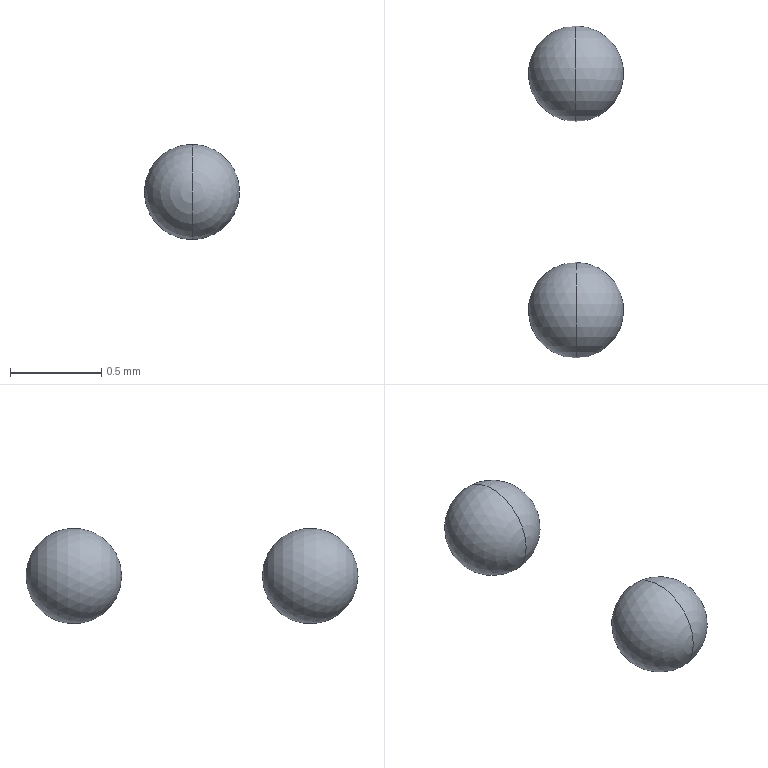Part | STEP file | COMPOUND | 2 solids | 4 faces | box 0.5247 x 1.822 x 0.5247 mm | volume 0.1513 mm3 | sphere 4
STEP:
#1=CARTESIAN_POINT('',(0.,0.,0.));
#2=DIRECTION('',(0.,0.,1.));
#3=DIRECTION('',(1.,0.,0.));
#4=AXIS2_PLACEMENT_3D('',#1,#2,#3);
#5=CARTESIAN_POINT('',(11.477,37.085,0.3471));
#6=VERTEX_POINT('',#5);
#7=CARTESIAN_POINT('',(11.477,37.61,0.3471));
#8=VERTEX_POINT('',#7);
#9=CARTESIAN_POINT('',(11.477,37.348,0.3471));
#10=DIRECTION('',(-1.,-0.000000175,0.));
#11=DIRECTION('',(0.000000175,-1.,0.));
#12=AXIS2_PLACEMENT_3D('',#9,#10,#11);
#13=CIRCLE('',#12,0.2623);
#14=CARTESIAN_POINT('',(11.477,37.348,0.3471));
#15=DIRECTION('',(-0.000000175,1.,0.));
#16=DIRECTION('',(0.,0.,1.));
#17=AXIS2_PLACEMENT_3D('',#14,#15,#16);
#18=SPHERICAL_SURFACE('',#17,0.2623);
#19=CARTESIAN_POINT('',(6.283,-1.571));
#20=CARTESIAN_POINT('',(6.283,-1.523));
#21=CARTESIAN_POINT('',(6.283,-1.428));
#22=CARTESIAN_POINT('',(6.283,-1.285));
#23=CARTESIAN_POINT('',(6.283,-1.142));
#24=CARTESIAN_POINT('',(6.283,-0.9996));
#25=CARTESIAN_POINT('',(6.283,-0.8568));
#26=CARTESIAN_POINT('',(6.283,-0.714));
#27=CARTESIAN_POINT('',(6.283,-0.5712));
#28=CARTESIAN_POINT('',(6.283,-0.4284));
#29=CARTESIAN_POINT('',(6.283,-0.2856));
#30=CARTESIAN_POINT('',(6.283,-0.1428));
#31=CARTESIAN_POINT('',(6.283,0.));
#32=CARTESIAN_POINT('',(6.283,0.1428));
#33=CARTESIAN_POINT('',(6.283,0.2856));
#34=CARTESIAN_POINT('',(6.283,0.4284));
#35=CARTESIAN_POINT('',(6.283,0.5712));
#36=CARTESIAN_POINT('',(6.283,0.714));
#37=CARTESIAN_POINT('',(6.283,0.8568));
#38=CARTESIAN_POINT('',(6.283,0.9996));
#39=CARTESIAN_POINT('',(6.283,1.142));
#40=CARTESIAN_POINT('',(6.283,1.285));
#41=CARTESIAN_POINT('',(6.283,1.428));
#42=CARTESIAN_POINT('',(6.283,1.523));
#43=CARTESIAN_POINT('',(6.283,1.571));
#44=B_SPLINE_CURVE_WITH_KNOTS('',3,(#19,#20,#21,#22,#23,#24,#25,#26,#27,#28,#29,#30,#31,#32,#33,#34,#35,#36,#37,#38,#39,#40,#41,#42,#43),.UNSPECIFIED.,.F.,.F.,(4,1,1,1,1,1,1,1,1,1,1,1,1,1,1,1,1,1,1,1,1,1,4),(0.,0.1428,0.2856,0.4284,0.5712,0.714,0.8568,0.9996,1.142,1.285,1.428,1.571,1.714,1.856,1.999,2.142,2.285,2.428,2.57,2.713,2.856,2.999,3.142),.QUASI_UNIFORM_KNOTS.);
#45=(GEOMETRIC_REPRESENTATION_CONTEXT(2)PARAMETRIC_REPRESENTATION_CONTEXT()REPRESENTATION_CONTEXT('',''));
#46=DEFINITIONAL_REPRESENTATION('',(#44),#45);
#47=PCURVE('',#18,#46);
#48=CARTESIAN_POINT('',(11.477,37.348,0.3471));
#49=DIRECTION('',(-0.000000175,1.,0.));
#50=DIRECTION('',(0.,0.,1.));
#51=AXIS2_PLACEMENT_3D('',#48,#49,#50);
#52=SPHERICAL_SURFACE('',#51,0.2623);
#53=CARTESIAN_POINT('',(0.,-1.571));
#54=CARTESIAN_POINT('',(0.,-1.523));
#55=CARTESIAN_POINT('',(0.,-1.428));
#56=CARTESIAN_POINT('',(0.,-1.285));
#57=CARTESIAN_POINT('',(0.,-1.142));
#58=CARTESIAN_POINT('',(0.,-0.9996));
#59=CARTESIAN_POINT('',(0.,-0.8568));
#60=CARTESIAN_POINT('',(0.,-0.714));
#61=CARTESIAN_POINT('',(0.,-0.5712));
#62=CARTESIAN_POINT('',(0.,-0.4284));
#63=CARTESIAN_POINT('',(0.,-0.2856));
#64=CARTESIAN_POINT('',(0.,-0.1428));
#65=CARTESIAN_POINT('',(0.,0.));
#66=CARTESIAN_POINT('',(0.,0.1428));
#67=CARTESIAN_POINT('',(0.,0.2856));
#68=CARTESIAN_POINT('',(0.,0.4284));
#69=CARTESIAN_POINT('',(0.,0.5712));
#70=CARTESIAN_POINT('',(0.,0.714));
#71=CARTESIAN_POINT('',(0.,0.8568));
#72=CARTESIAN_POINT('',(0.,0.9996));
#73=CARTESIAN_POINT('',(0.,1.142));
#74=CARTESIAN_POINT('',(0.,1.285));
#75=CARTESIAN_POINT('',(0.,1.428));
#76=CARTESIAN_POINT('',(0.,1.523));
#77=CARTESIAN_POINT('',(0.,1.571));
#78=B_SPLINE_CURVE_WITH_KNOTS('',3,(#53,#54,#55,#56,#57,#58,#59,#60,#61,#62,#63,#64,#65,#66,#67,#68,#69,#70,#71,#72,#73,#74,#75,#76,#77),.UNSPECIFIED.,.F.,.F.,(4,1,1,1,1,1,1,1,1,1,1,1,1,1,1,1,1,1,1,1,1,1,4),(0.,0.1428,0.2856,0.4284,0.5712,0.714,0.8568,0.9996,1.142,1.285,1.428,1.571,1.714,1.856,1.999,2.142,2.285,2.428,2.57,2.713,2.856,2.999,3.142),.QUASI_UNIFORM_KNOTS.);
#79=(GEOMETRIC_REPRESENTATION_CONTEXT(2)PARAMETRIC_REPRESENTATION_CONTEXT()REPRESENTATION_CONTEXT('',''));
#80=DEFINITIONAL_REPRESENTATION('',(#78),#79);
#81=PCURVE('',#52,#80);
#82=SURFACE_CURVE('',#13,(#47,#81),.PCURVE_S1.);
#83=EDGE_CURVE('',#6,#8,#82,.T.);
#84=ORIENTED_EDGE('',*,*,#83,.T.);
#85=CARTESIAN_POINT('',(11.477,37.348,0.3471));
#86=DIRECTION('',(1.,0.000000175,0.));
#87=DIRECTION('',(0.000000175,-1.,0.));
#88=AXIS2_PLACEMENT_3D('',#85,#86,#87);
#89=CIRCLE('',#88,0.2623);
#90=CARTESIAN_POINT('',(3.142,-1.571));
#91=CARTESIAN_POINT('',(3.142,-1.523));
#92=CARTESIAN_POINT('',(3.142,-1.428));
#93=CARTESIAN_POINT('',(3.142,-1.285));
#94=CARTESIAN_POINT('',(3.142,-1.142));
#95=CARTESIAN_POINT('',(3.142,-0.9996));
#96=CARTESIAN_POINT('',(3.142,-0.8568));
#97=CARTESIAN_POINT('',(3.142,-0.714));
#98=CARTESIAN_POINT('',(3.142,-0.5712));
#99=CARTESIAN_POINT('',(3.142,-0.4284));
#100=CARTESIAN_POINT('',(3.142,-0.2856));
#101=CARTESIAN_POINT('',(3.142,-0.1428));
#102=CARTESIAN_POINT('',(3.142,0.));
#103=CARTESIAN_POINT('',(3.142,0.1428));
#104=CARTESIAN_POINT('',(3.142,0.2856));
#105=CARTESIAN_POINT('',(3.142,0.4284));
#106=CARTESIAN_POINT('',(3.142,0.5712));
#107=CARTESIAN_POINT('',(3.142,0.714));
#108=CARTESIAN_POINT('',(3.142,0.8568));
#109=CARTESIAN_POINT('',(3.142,0.9996));
#110=CARTESIAN_POINT('',(3.142,1.142));
#111=CARTESIAN_POINT('',(3.142,1.285));
#112=CARTESIAN_POINT('',(3.142,1.428));
#113=CARTESIAN_POINT('',(3.142,1.523));
#114=CARTESIAN_POINT('',(3.142,1.571));
#115=B_SPLINE_CURVE_WITH_KNOTS('',3,(#90,#91,#92,#93,#94,#95,#96,#97,#98,#99,#100,#101,#102,#103,#104,#105,#106,#107,#108,#109,#110,#111,#112,#113,#114),.UNSPECIFIED.,.F.,.F.,(4,1,1,1,1,1,1,1,1,1,1,1,1,1,1,1,1,1,1,1,1,1,4),(0.,0.1428,0.2856,0.4284,0.5712,0.714,0.8568,0.9996,1.142,1.285,1.428,1.571,1.714,1.856,1.999,2.142,2.285,2.428,2.57,2.713,2.856,2.999,3.142),.QUASI_UNIFORM_KNOTS.);
#116=(GEOMETRIC_REPRESENTATION_CONTEXT(2)PARAMETRIC_REPRESENTATION_CONTEXT()REPRESENTATION_CONTEXT('',''));
#117=DEFINITIONAL_REPRESENTATION('',(#115),#116);
#118=PCURVE('',#18,#117);
#119=CARTESIAN_POINT('',(3.142,-1.571));
#120=CARTESIAN_POINT('',(3.142,-1.523));
#121=CARTESIAN_POINT('',(3.142,-1.428));
#122=CARTESIAN_POINT('',(3.142,-1.285));
#123=CARTESIAN_POINT('',(3.142,-1.142));
#124=CARTESIAN_POINT('',(3.142,-0.9996));
#125=CARTESIAN_POINT('',(3.142,-0.8568));
#126=CARTESIAN_POINT('',(3.142,-0.714));
#127=CARTESIAN_POINT('',(3.142,-0.5712));
#128=CARTESIAN_POINT('',(3.142,-0.4284));
#129=CARTESIAN_POINT('',(3.142,-0.2856));
#130=CARTESIAN_POINT('',(3.142,-0.1428));
#131=CARTESIAN_POINT('',(3.142,0.));
#132=CARTESIAN_POINT('',(3.142,0.1428));
#133=CARTESIAN_POINT('',(3.142,0.2856));
#134=CARTESIAN_POINT('',(3.142,0.4284));
#135=CARTESIAN_POINT('',(3.142,0.5712));
#136=CARTESIAN_POINT('',(3.142,0.714));
#137=CARTESIAN_POINT('',(3.142,0.8568));
#138=CARTESIAN_POINT('',(3.142,0.9996));
#139=CARTESIAN_POINT('',(3.142,1.142));
#140=CARTESIAN_POINT('',(3.142,1.285));
#141=CARTESIAN_POINT('',(3.142,1.428));
#142=CARTESIAN_POINT('',(3.142,1.523));
#143=CARTESIAN_POINT('',(3.142,1.571));
#144=B_SPLINE_CURVE_WITH_KNOTS('',3,(#119,#120,#121,#122,#123,#124,#125,#126,#127,#128,#129,#130,#131,#132,#133,#134,#135,#136,#137,#138,#139,#140,#141,#142,#143),.UNSPECIFIED.,.F.,.F.,(4,1,1,1,1,1,1,1,1,1,1,1,1,1,1,1,1,1,1,1,1,1,4),(0.,0.1428,0.2856,0.4284,0.5712,0.714,0.8568,0.9996,1.142,1.285,1.428,1.571,1.714,1.856,1.999,2.142,2.285,2.428,2.57,2.713,2.856,2.999,3.142),.QUASI_UNIFORM_KNOTS.);
#145=(GEOMETRIC_REPRESENTATION_CONTEXT(2)PARAMETRIC_REPRESENTATION_CONTEXT()REPRESENTATION_CONTEXT('',''));
#146=DEFINITIONAL_REPRESENTATION('',(#144),#145);
#147=PCURVE('',#52,#146);
#148=SURFACE_CURVE('',#89,(#118,#147),.PCURVE_S1.);
#149=EDGE_CURVE('',#6,#8,#148,.T.);
#150=ORIENTED_EDGE('',*,*,#149,.F.);
#151=EDGE_LOOP('',(#84,#150));
#152=FACE_BOUND('',#151,.T.);
#153=ADVANCED_FACE('',(#152),#18,.T.);
#154=ORIENTED_EDGE('',*,*,#149,.T.);
#155=ORIENTED_EDGE('',*,*,#83,.F.);
#156=EDGE_LOOP('',(#154,#155));
#157=FACE_BOUND('',#156,.T.);
#158=ADVANCED_FACE('',(#157),#52,.T.);
#159=CLOSED_SHELL('',(#153,#158));
#160=MANIFOLD_SOLID_BREP('',#159);
#161=CARTESIAN_POINT('',(11.477,35.788,0.3471));
#162=VERTEX_POINT('',#161);
#163=CARTESIAN_POINT('',(11.477,36.313,0.3471));
#164=VERTEX_POINT('',#163);
#165=CARTESIAN_POINT('',(11.477,36.051,0.3471));
#166=DIRECTION('',(-1.,-0.000000175,0.));
#167=DIRECTION('',(0.000000175,-1.,0.));
#168=AXIS2_PLACEMENT_3D('',#165,#166,#167);
#169=CIRCLE('',#168,0.2623);
#170=CARTESIAN_POINT('',(11.477,36.051,0.3471));
#171=DIRECTION('',(-0.000000175,1.,0.));
#172=DIRECTION('',(0.,0.,1.));
#173=AXIS2_PLACEMENT_3D('',#170,#171,#172);
#174=SPHERICAL_SURFACE('',#173,0.2623);
#175=CARTESIAN_POINT('',(6.283,-1.571));
#176=CARTESIAN_POINT('',(6.283,-1.523));
#177=CARTESIAN_POINT('',(6.283,-1.428));
#178=CARTESIAN_POINT('',(6.283,-1.285));
#179=CARTESIAN_POINT('',(6.283,-1.142));
#180=CARTESIAN_POINT('',(6.283,-0.9996));
#181=CARTESIAN_POINT('',(6.283,-0.8568));
#182=CARTESIAN_POINT('',(6.283,-0.714));
#183=CARTESIAN_POINT('',(6.283,-0.5712));
#184=CARTESIAN_POINT('',(6.283,-0.4284));
#185=CARTESIAN_POINT('',(6.283,-0.2856));
#186=CARTESIAN_POINT('',(6.283,-0.1428));
#187=CARTESIAN_POINT('',(6.283,0.));
#188=CARTESIAN_POINT('',(6.283,0.1428));
#189=CARTESIAN_POINT('',(6.283,0.2856));
#190=CARTESIAN_POINT('',(6.283,0.4284));
#191=CARTESIAN_POINT('',(6.283,0.5712));
#192=CARTESIAN_POINT('',(6.283,0.714));
#193=CARTESIAN_POINT('',(6.283,0.8568));
#194=CARTESIAN_POINT('',(6.283,0.9996));
#195=CARTESIAN_POINT('',(6.283,1.142));
#196=CARTESIAN_POINT('',(6.283,1.285));
#197=CARTESIAN_POINT('',(6.283,1.428));
#198=CARTESIAN_POINT('',(6.283,1.523));
#199=CARTESIAN_POINT('',(6.283,1.571));
#200=B_SPLINE_CURVE_WITH_KNOTS('',3,(#175,#176,#177,#178,#179,#180,#181,#182,#183,#184,#185,#186,#187,#188,#189,#190,#191,#192,#193,#194,#195,#196,#197,#198,#199),.UNSPECIFIED.,.F.,.F.,(4,1,1,1,1,1,1,1,1,1,1,1,1,1,1,1,1,1,1,1,1,1,4),(0.,0.1428,0.2856,0.4284,0.5712,0.714,0.8568,0.9996,1.142,1.285,1.428,1.571,1.714,1.856,1.999,2.142,2.285,2.428,2.57,2.713,2.856,2.999,3.142),.QUASI_UNIFORM_KNOTS.);
#201=(GEOMETRIC_REPRESENTATION_CONTEXT(2)PARAMETRIC_REPRESENTATION_CONTEXT()REPRESENTATION_CONTEXT('',''));
#202=DEFINITIONAL_REPRESENTATION('',(#200),#201);
#203=PCURVE('',#174,#202);
#204=CARTESIAN_POINT('',(11.477,36.051,0.3471));
#205=DIRECTION('',(-0.000000175,1.,0.));
#206=DIRECTION('',(0.,0.,1.));
#207=AXIS2_PLACEMENT_3D('',#204,#205,#206);
#208=SPHERICAL_SURFACE('',#207,0.2623);
#209=CARTESIAN_POINT('',(0.,-1.571));
#210=CARTESIAN_POINT('',(0.,-1.523));
#211=CARTESIAN_POINT('',(0.,-1.428));
#212=CARTESIAN_POINT('',(0.,-1.285));
#213=CARTESIAN_POINT('',(0.,-1.142));
#214=CARTESIAN_POINT('',(0.,-0.9996));
#215=CARTESIAN_POINT('',(0.,-0.8568));
#216=CARTESIAN_POINT('',(0.,-0.714));
#217=CARTESIAN_POINT('',(0.,-0.5712));
#218=CARTESIAN_POINT('',(0.,-0.4284));
#219=CARTESIAN_POINT('',(0.,-0.2856));
#220=CARTESIAN_POINT('',(0.,-0.1428));
#221=CARTESIAN_POINT('',(0.,0.));
#222=CARTESIAN_POINT('',(0.,0.1428));
#223=CARTESIAN_POINT('',(0.,0.2856));
#224=CARTESIAN_POINT('',(0.,0.4284));
#225=CARTESIAN_POINT('',(0.,0.5712));
#226=CARTESIAN_POINT('',(0.,0.714));
#227=CARTESIAN_POINT('',(0.,0.8568));
#228=CARTESIAN_POINT('',(0.,0.9996));
#229=CARTESIAN_POINT('',(0.,1.142));
#230=CARTESIAN_POINT('',(0.,1.285));
#231=CARTESIAN_POINT('',(0.,1.428));
#232=CARTESIAN_POINT('',(0.,1.523));
#233=CARTESIAN_POINT('',(0.,1.571));
#234=B_SPLINE_CURVE_WITH_KNOTS('',3,(#209,#210,#211,#212,#213,#214,#215,#216,#217,#218,#219,#220,#221,#222,#223,#224,#225,#226,#227,#228,#229,#230,#231,#232,#233),.UNSPECIFIED.,.F.,.F.,(4,1,1,1,1,1,1,1,1,1,1,1,1,1,1,1,1,1,1,1,1,1,4),(0.,0.1428,0.2856,0.4284,0.5712,0.714,0.8568,0.9996,1.142,1.285,1.428,1.571,1.714,1.856,1.999,2.142,2.285,2.428,2.57,2.713,2.856,2.999,3.142),.QUASI_UNIFORM_KNOTS.);
#235=(GEOMETRIC_REPRESENTATION_CONTEXT(2)PARAMETRIC_REPRESENTATION_CONTEXT()REPRESENTATION_CONTEXT('',''));
#236=DEFINITIONAL_REPRESENTATION('',(#234),#235);
#237=PCURVE('',#208,#236);
#238=SURFACE_CURVE('',#169,(#203,#237),.PCURVE_S1.);
#239=EDGE_CURVE('',#162,#164,#238,.T.);
#240=ORIENTED_EDGE('',*,*,#239,.T.);
#241=CARTESIAN_POINT('',(11.477,36.051,0.3471));
#242=DIRECTION('',(1.,0.000000175,0.));
#243=DIRECTION('',(0.000000175,-1.,0.));
#244=AXIS2_PLACEMENT_3D('',#241,#242,#243);
#245=CIRCLE('',#244,0.2623);
#246=CARTESIAN_POINT('',(3.142,-1.571));
#247=CARTESIAN_POINT('',(3.142,-1.523));
#248=CARTESIAN_POINT('',(3.142,-1.428));
#249=CARTESIAN_POINT('',(3.142,-1.285));
#250=CARTESIAN_POINT('',(3.142,-1.142));
#251=CARTESIAN_POINT('',(3.142,-0.9996));
#252=CARTESIAN_POINT('',(3.142,-0.8568));
#253=CARTESIAN_POINT('',(3.142,-0.714));
#254=CARTESIAN_POINT('',(3.142,-0.5712));
#255=CARTESIAN_POINT('',(3.142,-0.4284));
#256=CARTESIAN_POINT('',(3.142,-0.2856));
#257=CARTESIAN_POINT('',(3.142,-0.1428));
#258=CARTESIAN_POINT('',(3.142,0.));
#259=CARTESIAN_POINT('',(3.142,0.1428));
#260=CARTESIAN_POINT('',(3.142,0.2856));
#261=CARTESIAN_POINT('',(3.142,0.4284));
#262=CARTESIAN_POINT('',(3.142,0.5712));
#263=CARTESIAN_POINT('',(3.142,0.714));
#264=CARTESIAN_POINT('',(3.142,0.8568));
#265=CARTESIAN_POINT('',(3.142,0.9996));
#266=CARTESIAN_POINT('',(3.142,1.142));
#267=CARTESIAN_POINT('',(3.142,1.285));
#268=CARTESIAN_POINT('',(3.142,1.428));
#269=CARTESIAN_POINT('',(3.142,1.523));
#270=CARTESIAN_POINT('',(3.142,1.571));
#271=B_SPLINE_CURVE_WITH_KNOTS('',3,(#246,#247,#248,#249,#250,#251,#252,#253,#254,#255,#256,#257,#258,#259,#260,#261,#262,#263,#264,#265,#266,#267,#268,#269,#270),.UNSPECIFIED.,.F.,.F.,(4,1,1,1,1,1,1,1,1,1,1,1,1,1,1,1,1,1,1,1,1,1,4),(0.,0.1428,0.2856,0.4284,0.5712,0.714,0.8568,0.9996,1.142,1.285,1.428,1.571,1.714,1.856,1.999,2.142,2.285,2.428,2.57,2.713,2.856,2.999,3.142),.QUASI_UNIFORM_KNOTS.);
#272=(GEOMETRIC_REPRESENTATION_CONTEXT(2)PARAMETRIC_REPRESENTATION_CONTEXT()REPRESENTATION_CONTEXT('',''));
#273=DEFINITIONAL_REPRESENTATION('',(#271),#272);
#274=PCURVE('',#174,#273);
#275=CARTESIAN_POINT('',(3.142,-1.571));
#276=CARTESIAN_POINT('',(3.142,-1.523));
#277=CARTESIAN_POINT('',(3.142,-1.428));
#278=CARTESIAN_POINT('',(3.142,-1.285));
#279=CARTESIAN_POINT('',(3.142,-1.142));
#280=CARTESIAN_POINT('',(3.142,-0.9996));
#281=CARTESIAN_POINT('',(3.142,-0.8568));
#282=CARTESIAN_POINT('',(3.142,-0.714));
#283=CARTESIAN_POINT('',(3.142,-0.5712));
#284=CARTESIAN_POINT('',(3.142,-0.4284));
#285=CARTESIAN_POINT('',(3.142,-0.2856));
#286=CARTESIAN_POINT('',(3.142,-0.1428));
#287=CARTESIAN_POINT('',(3.142,0.));
#288=CARTESIAN_POINT('',(3.142,0.1428));
#289=CARTESIAN_POINT('',(3.142,0.2856));
#290=CARTESIAN_POINT('',(3.142,0.4284));
#291=CARTESIAN_POINT('',(3.142,0.5712));
#292=CARTESIAN_POINT('',(3.142,0.714));
#293=CARTESIAN_POINT('',(3.142,0.8568));
#294=CARTESIAN_POINT('',(3.142,0.9996));
#295=CARTESIAN_POINT('',(3.142,1.142));
#296=CARTESIAN_POINT('',(3.142,1.285));
#297=CARTESIAN_POINT('',(3.142,1.428));
#298=CARTESIAN_POINT('',(3.142,1.523));
#299=CARTESIAN_POINT('',(3.142,1.571));
#300=B_SPLINE_CURVE_WITH_KNOTS('',3,(#275,#276,#277,#278,#279,#280,#281,#282,#283,#284,#285,#286,#287,#288,#289,#290,#291,#292,#293,#294,#295,#296,#297,#298,#299),.UNSPECIFIED.,.F.,.F.,(4,1,1,1,1,1,1,1,1,1,1,1,1,1,1,1,1,1,1,1,1,1,4),(0.,0.1428,0.2856,0.4284,0.5712,0.714,0.8568,0.9996,1.142,1.285,1.428,1.571,1.714,1.856,1.999,2.142,2.285,2.428,2.57,2.713,2.856,2.999,3.142),.QUASI_UNIFORM_KNOTS.);
#301=(GEOMETRIC_REPRESENTATION_CONTEXT(2)PARAMETRIC_REPRESENTATION_CONTEXT()REPRESENTATION_CONTEXT('',''));
#302=DEFINITIONAL_REPRESENTATION('',(#300),#301);
#303=PCURVE('',#208,#302);
#304=SURFACE_CURVE('',#245,(#274,#303),.PCURVE_S1.);
#305=EDGE_CURVE('',#162,#164,#304,.T.);
#306=ORIENTED_EDGE('',*,*,#305,.F.);
#307=EDGE_LOOP('',(#240,#306));
#308=FACE_BOUND('',#307,.T.);
#309=ADVANCED_FACE('',(#308),#174,.T.);
#310=ORIENTED_EDGE('',*,*,#305,.T.);
#311=ORIENTED_EDGE('',*,*,#239,.F.);
#312=EDGE_LOOP('',(#310,#311));
#313=FACE_BOUND('',#312,.T.);
#314=ADVANCED_FACE('',(#313),#208,.T.);
#315=CLOSED_SHELL('',(#309,#314));
#316=MANIFOLD_SOLID_BREP('',#315);
#317=(LENGTH_UNIT()NAMED_UNIT(*)SI_UNIT(.MILLI.,.METRE.));
#318=UNCERTAINTY_MEASURE_WITH_UNIT(LENGTH_MEASURE(0.0000001),#317,'','');
#319=(NAMED_UNIT(*)PLANE_ANGLE_UNIT()SI_UNIT($,.RADIAN.));
#320=(NAMED_UNIT(*)SI_UNIT($,.STERADIAN.)SOLID_ANGLE_UNIT());
#321=(GEOMETRIC_REPRESENTATION_CONTEXT(3)GLOBAL_UNCERTAINTY_ASSIGNED_CONTEXT((#318))GLOBAL_UNIT_ASSIGNED_CONTEXT((#317,#319,#320))REPRESENTATION_CONTEXT('',''));
#322=SHAPE_REPRESENTATION('',(#4,#160,#316),#321);